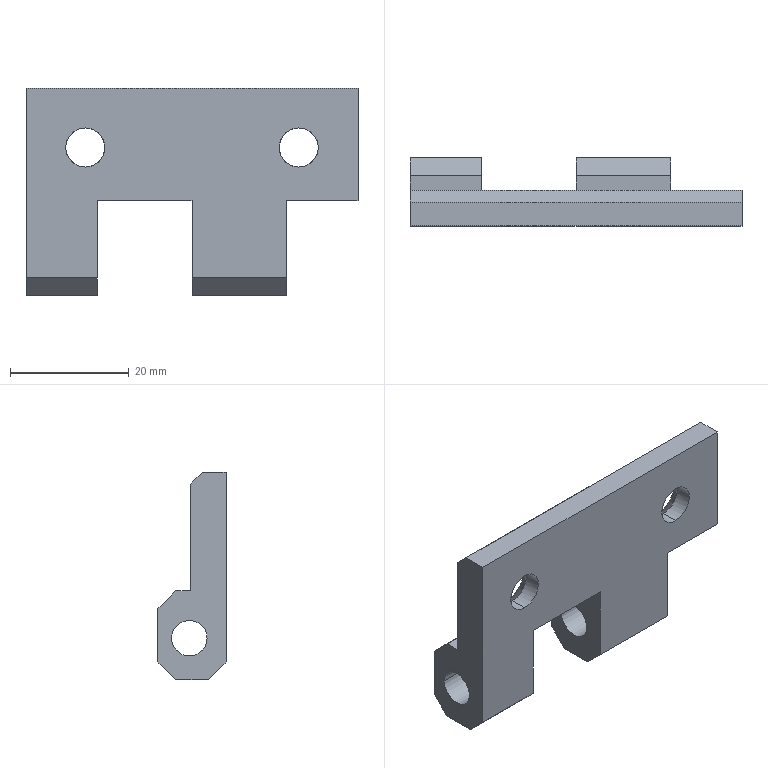Part | NX | features solid 2 | 1 solid | 35 faces | box 56 x 11.5 x 35 mm | volume 9428 mm3 | plane 23 | cylinder 8 | cone 4 | commonest cylinder face diameters 6 x4 6.6 x4
STEP:
#1=CARTESIAN_POINT('',(-668.,-707.,1288.));
#2=VERTEX_POINT('',#1);
#3=CARTESIAN_POINT('',(-668.,-710.,1291.));
#4=VERTEX_POINT('',#3);
#5=CARTESIAN_POINT('',(-668.,-710.,1291.));
#6=DIRECTION('',(0.,-0.7071,0.7071));
#7=VECTOR('',#6,1000.);
#8=LINE('',#5,#7);
#9=EDGE_CURVE('',#2,#4,#8,.T.);
#10=ORIENTED_EDGE('',*,*,#9,.F.);
#11=CARTESIAN_POINT('',(-652.,-707.,1288.));
#12=VERTEX_POINT('',#11);
#13=CARTESIAN_POINT('',(-696.,-707.,1288.));
#14=DIRECTION('',(-1.,0.,0.));
#15=VECTOR('',#14,1000.);
#16=LINE('',#13,#15);
#17=EDGE_CURVE('',#12,#2,#16,.T.);
#18=ORIENTED_EDGE('',*,*,#17,.F.);
#19=CARTESIAN_POINT('',(-652.,-710.,1291.));
#20=VERTEX_POINT('',#19);
#21=CARTESIAN_POINT('',(-652.,-710.,1291.));
#22=DIRECTION('',(0.,0.7071,-0.7071));
#23=VECTOR('',#22,1000.);
#24=LINE('',#21,#23);
#25=EDGE_CURVE('',#20,#12,#24,.T.);
#26=ORIENTED_EDGE('',*,*,#25,.F.);
#27=CARTESIAN_POINT('',(-696.,-710.,1291.));
#28=DIRECTION('',(1.,0.,0.));
#29=VECTOR('',#28,1000.);
#30=LINE('',#27,#29);
#31=EDGE_CURVE('',#4,#20,#30,.T.);
#32=ORIENTED_EDGE('',*,*,#31,.F.);
#33=EDGE_LOOP('',(#10,#18,#26,#32));
#34=FACE_BOUND('',#33,.T.);
#35=CARTESIAN_POINT('',(-696.,-710.,1291.));
#36=DIRECTION('',(0.,0.7071,0.7071));
#37=DIRECTION('',(1.,0.,0.));
#38=AXIS2_PLACEMENT_3D('',#35,#36,#37);
#39=PLANE('',#38);
#40=ADVANCED_FACE('',(#34),#39,.F.);
#41=CARTESIAN_POINT('',(-696.,-707.,1288.));
#42=VERTEX_POINT('',#41);
#43=CARTESIAN_POINT('',(-696.,-710.,1291.));
#44=VERTEX_POINT('',#43);
#45=CARTESIAN_POINT('',(-696.,-710.,1291.));
#46=DIRECTION('',(0.,-0.7071,0.7071));
#47=VECTOR('',#46,1000.);
#48=LINE('',#45,#47);
#49=EDGE_CURVE('',#42,#44,#48,.T.);
#50=ORIENTED_EDGE('',*,*,#49,.F.);
#51=CARTESIAN_POINT('',(-684.,-707.,1288.));
#52=VERTEX_POINT('',#51);
#53=CARTESIAN_POINT('',(-696.,-707.,1288.));
#54=DIRECTION('',(-1.,0.,0.));
#55=VECTOR('',#54,1000.);
#56=LINE('',#53,#55);
#57=EDGE_CURVE('',#52,#42,#56,.T.);
#58=ORIENTED_EDGE('',*,*,#57,.F.);
#59=CARTESIAN_POINT('',(-684.,-710.,1291.));
#60=VERTEX_POINT('',#59);
#61=CARTESIAN_POINT('',(-684.,-710.,1291.));
#62=DIRECTION('',(0.,0.7071,-0.7071));
#63=VECTOR('',#62,1000.);
#64=LINE('',#61,#63);
#65=EDGE_CURVE('',#60,#52,#64,.T.);
#66=ORIENTED_EDGE('',*,*,#65,.F.);
#67=CARTESIAN_POINT('',(-696.,-710.,1291.));
#68=DIRECTION('',(1.,0.,0.));
#69=VECTOR('',#68,1000.);
#70=LINE('',#67,#69);
#71=EDGE_CURVE('',#44,#60,#70,.T.);
#72=ORIENTED_EDGE('',*,*,#71,.F.);
#73=EDGE_LOOP('',(#50,#58,#66,#72));
#74=FACE_BOUND('',#73,.T.);
#75=CARTESIAN_POINT('',(-696.,-710.,1291.));
#76=DIRECTION('',(0.,0.7071,0.7071));
#77=DIRECTION('',(1.,0.,0.));
#78=AXIS2_PLACEMENT_3D('',#75,#76,#77);
#79=PLANE('',#78);
#80=ADVANCED_FACE('',(#74),#79,.F.);
#81=CARTESIAN_POINT('',(-668.,-701.5,1288.));
#82=VERTEX_POINT('',#81);
#83=CARTESIAN_POINT('',(-668.,-698.5,1291.));
#84=VERTEX_POINT('',#83);
#85=CARTESIAN_POINT('',(-668.,-725.516,1263.984));
#86=DIRECTION('',(0.,0.7071,0.7071));
#87=VECTOR('',#86,1000.);
#88=LINE('',#85,#87);
#89=EDGE_CURVE('',#82,#84,#88,.T.);
#90=ORIENTED_EDGE('',*,*,#89,.T.);
#91=CARTESIAN_POINT('',(-652.,-698.5,1291.));
#92=VERTEX_POINT('',#91);
#93=CARTESIAN_POINT('',(-719.032,-698.5,1291.));
#94=DIRECTION('',(1.,0.,0.));
#95=VECTOR('',#94,1000.);
#96=LINE('',#93,#95);
#97=EDGE_CURVE('',#84,#92,#96,.T.);
#98=ORIENTED_EDGE('',*,*,#97,.T.);
#99=CARTESIAN_POINT('',(-652.,-701.5,1288.));
#100=VERTEX_POINT('',#99);
#101=CARTESIAN_POINT('',(-652.,-698.5,1291.));
#102=DIRECTION('',(0.,0.7071,0.7071));
#103=VECTOR('',#102,1000.);
#104=LINE('',#101,#103);
#105=EDGE_CURVE('',#100,#92,#104,.T.);
#106=ORIENTED_EDGE('',*,*,#105,.F.);
#107=CARTESIAN_POINT('',(-696.,-701.5,1288.));
#108=DIRECTION('',(1.,0.,0.));
#109=VECTOR('',#108,1000.);
#110=LINE('',#107,#109);
#111=EDGE_CURVE('',#82,#100,#110,.T.);
#112=ORIENTED_EDGE('',*,*,#111,.F.);
#113=EDGE_LOOP('',(#90,#98,#106,#112));
#114=FACE_BOUND('',#113,.T.);
#115=CARTESIAN_POINT('',(-719.032,-698.5,1291.));
#116=DIRECTION('',(0.,0.7071,-0.7071));
#117=DIRECTION('',(-1.,0.,0.));
#118=AXIS2_PLACEMENT_3D('',#115,#116,#117);
#119=PLANE('',#118);
#120=ADVANCED_FACE('',(#114),#119,.T.);
#121=CARTESIAN_POINT('',(-696.,-701.5,1288.));
#122=VERTEX_POINT('',#121);
#123=CARTESIAN_POINT('',(-696.,-698.5,1291.));
#124=VERTEX_POINT('',#123);
#125=CARTESIAN_POINT('',(-696.,-688.25,1301.25));
#126=DIRECTION('',(0.,0.7071,0.7071));
#127=VECTOR('',#126,1000.);
#128=LINE('',#125,#127);
#129=EDGE_CURVE('',#122,#124,#128,.T.);
#130=ORIENTED_EDGE('',*,*,#129,.T.);
#131=CARTESIAN_POINT('',(-684.,-698.5,1291.));
#132=VERTEX_POINT('',#131);
#133=CARTESIAN_POINT('',(-719.032,-698.5,1291.));
#134=DIRECTION('',(1.,0.,0.));
#135=VECTOR('',#134,1000.);
#136=LINE('',#133,#135);
#137=EDGE_CURVE('',#124,#132,#136,.T.);
#138=ORIENTED_EDGE('',*,*,#137,.T.);
#139=CARTESIAN_POINT('',(-684.,-701.5,1288.));
#140=VERTEX_POINT('',#139);
#141=CARTESIAN_POINT('',(-684.,-733.516,1255.984));
#142=DIRECTION('',(0.,-0.7071,-0.7071));
#143=VECTOR('',#142,1000.);
#144=LINE('',#141,#143);
#145=EDGE_CURVE('',#132,#140,#144,.T.);
#146=ORIENTED_EDGE('',*,*,#145,.T.);
#147=CARTESIAN_POINT('',(-719.032,-701.5,1288.));
#148=DIRECTION('',(1.,0.,0.));
#149=VECTOR('',#148,1000.);
#150=LINE('',#147,#149);
#151=EDGE_CURVE('',#122,#140,#150,.T.);
#152=ORIENTED_EDGE('',*,*,#151,.F.);
#153=EDGE_LOOP('',(#130,#138,#146,#152));
#154=FACE_BOUND('',#153,.T.);
#155=CARTESIAN_POINT('',(-719.032,-698.5,1291.));
#156=DIRECTION('',(0.,0.7071,-0.7071));
#157=DIRECTION('',(-1.,0.,0.));
#158=AXIS2_PLACEMENT_3D('',#155,#156,#157);
#159=PLANE('',#158);
#160=ADVANCED_FACE('',(#154),#159,.T.);
#161=CARTESIAN_POINT('',(-668.,-698.5,1300.));
#162=VERTEX_POINT('',#161);
#163=CARTESIAN_POINT('',(-668.,-701.5,1303.));
#164=VERTEX_POINT('',#163);
#165=CARTESIAN_POINT('',(-668.,-734.016,1335.516));
#166=DIRECTION('',(0.,-0.7071,0.7071));
#167=VECTOR('',#166,1000.);
#168=LINE('',#165,#167);
#169=EDGE_CURVE('',#162,#164,#168,.T.);
#170=ORIENTED_EDGE('',*,*,#169,.T.);
#171=CARTESIAN_POINT('',(-652.,-701.5,1303.));
#172=VERTEX_POINT('',#171);
#173=CARTESIAN_POINT('',(-719.032,-701.5,1303.));
#174=DIRECTION('',(1.,0.,0.));
#175=VECTOR('',#174,1000.);
#176=LINE('',#173,#175);
#177=EDGE_CURVE('',#164,#172,#176,.T.);
#178=ORIENTED_EDGE('',*,*,#177,.T.);
#179=CARTESIAN_POINT('',(-652.,-698.5,1300.));
#180=VERTEX_POINT('',#179);
#181=CARTESIAN_POINT('',(-652.,-701.5,1303.));
#182=DIRECTION('',(0.,-0.7071,0.7071));
#183=VECTOR('',#182,1000.);
#184=LINE('',#181,#183);
#185=EDGE_CURVE('',#180,#172,#184,.T.);
#186=ORIENTED_EDGE('',*,*,#185,.F.);
#187=CARTESIAN_POINT('',(-719.032,-698.5,1300.));
#188=DIRECTION('',(1.,0.,0.));
#189=VECTOR('',#188,1000.);
#190=LINE('',#187,#189);
#191=EDGE_CURVE('',#162,#180,#190,.T.);
#192=ORIENTED_EDGE('',*,*,#191,.F.);
#193=EDGE_LOOP('',(#170,#178,#186,#192));
#194=FACE_BOUND('',#193,.T.);
#195=CARTESIAN_POINT('',(-719.032,-701.5,1303.));
#196=DIRECTION('',(0.,0.7071,0.7071));
#197=DIRECTION('',(1.,0.,0.));
#198=AXIS2_PLACEMENT_3D('',#195,#196,#197);
#199=PLANE('',#198);
#200=ADVANCED_FACE('',(#194),#199,.T.);
#201=CARTESIAN_POINT('',(-696.,-698.5,1300.));
#202=VERTEX_POINT('',#201);
#203=CARTESIAN_POINT('',(-696.,-701.5,1303.));
#204=VERTEX_POINT('',#203);
#205=CARTESIAN_POINT('',(-696.,-715.75,1317.25));
#206=DIRECTION('',(0.,-0.7071,0.7071));
#207=VECTOR('',#206,1000.);
#208=LINE('',#205,#207);
#209=EDGE_CURVE('',#202,#204,#208,.T.);
#210=ORIENTED_EDGE('',*,*,#209,.T.);
#211=CARTESIAN_POINT('',(-684.,-701.5,1303.));
#212=VERTEX_POINT('',#211);
#213=CARTESIAN_POINT('',(-719.032,-701.5,1303.));
#214=DIRECTION('',(1.,0.,0.));
#215=VECTOR('',#214,1000.);
#216=LINE('',#213,#215);
#217=EDGE_CURVE('',#204,#212,#216,.T.);
#218=ORIENTED_EDGE('',*,*,#217,.T.);
#219=CARTESIAN_POINT('',(-684.,-698.5,1300.));
#220=VERTEX_POINT('',#219);
#221=CARTESIAN_POINT('',(-684.,-726.016,1327.516));
#222=DIRECTION('',(0.,0.7071,-0.7071));
#223=VECTOR('',#222,1000.);
#224=LINE('',#221,#223);
#225=EDGE_CURVE('',#212,#220,#224,.T.);
#226=ORIENTED_EDGE('',*,*,#225,.T.);
#227=CARTESIAN_POINT('',(-719.032,-698.5,1300.));
#228=DIRECTION('',(1.,0.,0.));
#229=VECTOR('',#228,1000.);
#230=LINE('',#227,#229);
#231=EDGE_CURVE('',#202,#220,#230,.T.);
#232=ORIENTED_EDGE('',*,*,#231,.F.);
#233=EDGE_LOOP('',(#210,#218,#226,#232));
#234=FACE_BOUND('',#233,.T.);
#235=CARTESIAN_POINT('',(-719.032,-701.5,1303.));
#236=DIRECTION('',(0.,0.7071,0.7071));
#237=DIRECTION('',(1.,0.,0.));
#238=AXIS2_PLACEMENT_3D('',#235,#236,#237);
#239=PLANE('',#238);
#240=ADVANCED_FACE('',(#234),#239,.T.);
#241=CARTESIAN_POINT('',(-684.,-700.8,1295.));
#242=VERTEX_POINT('',#241);
#243=CARTESIAN_POINT('',(-696.,-700.8,1295.));
#244=VERTEX_POINT('',#243);
#245=CARTESIAN_POINT('',(-640.,-700.8,1295.));
#246=DIRECTION('',(-1.,0.,0.));
#247=VECTOR('',#246,1000.);
#248=LINE('',#245,#247);
#249=EDGE_CURVE('',#242,#244,#248,.T.);
#250=ORIENTED_EDGE('',*,*,#249,.F.);
#251=CARTESIAN_POINT('',(-684.,-706.8,1295.));
#252=VERTEX_POINT('',#251);
#253=CARTESIAN_POINT('',(-684.,-703.8,1295.));
#254=DIRECTION('',(-1.,0.,0.));
#255=DIRECTION('',(0.,0.,1.));
#256=AXIS2_PLACEMENT_3D('',#253,#254,#255);
#257=CIRCLE('',#256,3.);
#258=EDGE_CURVE('',#252,#242,#257,.T.);
#259=ORIENTED_EDGE('',*,*,#258,.F.);
#260=CARTESIAN_POINT('',(-696.,-706.8,1295.));
#261=VERTEX_POINT('',#260);
#262=CARTESIAN_POINT('',(-640.,-706.8,1295.));
#263=DIRECTION('',(-1.,0.,0.));
#264=VECTOR('',#263,1000.);
#265=LINE('',#262,#264);
#266=EDGE_CURVE('',#261,#252,#265,.F.);
#267=ORIENTED_EDGE('',*,*,#266,.F.);
#268=CARTESIAN_POINT('',(-696.,-703.8,1295.));
#269=DIRECTION('',(1.,0.,0.));
#270=DIRECTION('',(0.,-1.,0.));
#271=AXIS2_PLACEMENT_3D('',#268,#269,#270);
#272=CIRCLE('',#271,3.);
#273=EDGE_CURVE('',#244,#261,#272,.T.);
#274=ORIENTED_EDGE('',*,*,#273,.F.);
#275=EDGE_LOOP('',(#250,#259,#267,#274));
#276=FACE_BOUND('',#275,.T.);
#277=CARTESIAN_POINT('',(-640.,-703.8,1295.));
#278=DIRECTION('',(-1.,0.,0.));
#279=DIRECTION('',(0.,-1.,0.));
#280=AXIS2_PLACEMENT_3D('',#277,#278,#279);
#281=CYLINDRICAL_SURFACE('',#280,3.);
#282=ADVANCED_FACE('',(#276),#281,.F.);
#283=CARTESIAN_POINT('',(-668.,-700.8,1295.));
#284=VERTEX_POINT('',#283);
#285=CARTESIAN_POINT('',(-652.,-700.8,1295.));
#286=VERTEX_POINT('',#285);
#287=CARTESIAN_POINT('',(-640.,-700.8,1295.));
#288=DIRECTION('',(-1.,0.,0.));
#289=VECTOR('',#288,1000.);
#290=LINE('',#287,#289);
#291=EDGE_CURVE('',#284,#286,#290,.F.);
#292=ORIENTED_EDGE('',*,*,#291,.T.);
#293=CARTESIAN_POINT('',(-652.,-706.8,1295.));
#294=VERTEX_POINT('',#293);
#295=CARTESIAN_POINT('',(-652.,-703.8,1295.));
#296=DIRECTION('',(-1.,0.,0.));
#297=DIRECTION('',(0.,0.,1.));
#298=AXIS2_PLACEMENT_3D('',#295,#296,#297);
#299=CIRCLE('',#298,3.);
#300=EDGE_CURVE('',#294,#286,#299,.T.);
#301=ORIENTED_EDGE('',*,*,#300,.F.);
#302=CARTESIAN_POINT('',(-668.,-706.8,1295.));
#303=VERTEX_POINT('',#302);
#304=CARTESIAN_POINT('',(-640.,-706.8,1295.));
#305=DIRECTION('',(-1.,0.,0.));
#306=VECTOR('',#305,1000.);
#307=LINE('',#304,#306);
#308=EDGE_CURVE('',#294,#303,#307,.T.);
#309=ORIENTED_EDGE('',*,*,#308,.T.);
#310=CARTESIAN_POINT('',(-668.,-703.8,1295.));
#311=DIRECTION('',(1.,0.,0.));
#312=DIRECTION('',(0.,-1.,0.));
#313=AXIS2_PLACEMENT_3D('',#310,#311,#312);
#314=CIRCLE('',#313,3.);
#315=EDGE_CURVE('',#284,#303,#314,.T.);
#316=ORIENTED_EDGE('',*,*,#315,.F.);
#317=EDGE_LOOP('',(#292,#301,#309,#316));
#318=FACE_BOUND('',#317,.T.);
#319=CARTESIAN_POINT('',(-640.,-703.8,1295.));
#320=DIRECTION('',(-1.,0.,0.));
#321=DIRECTION('',(0.,-1.,0.));
#322=AXIS2_PLACEMENT_3D('',#319,#320,#321);
#323=CYLINDRICAL_SURFACE('',#322,3.);
#324=ADVANCED_FACE('',(#318),#323,.F.);
#325=CARTESIAN_POINT('',(-668.,-710.,1304.));
#326=VERTEX_POINT('',#325);
#327=CARTESIAN_POINT('',(-684.,-710.,1304.));
#328=VERTEX_POINT('',#327);
#329=CARTESIAN_POINT('',(-696.,-710.,1304.));
#330=DIRECTION('',(-1.,0.,0.));
#331=VECTOR('',#330,1000.);
#332=LINE('',#329,#331);
#333=EDGE_CURVE('',#326,#328,#332,.T.);
#334=ORIENTED_EDGE('',*,*,#333,.T.);
#335=CARTESIAN_POINT('',(-684.,-704.,1304.));
#336=VERTEX_POINT('',#335);
#337=CARTESIAN_POINT('',(-684.,-765.532,1304.));
#338=DIRECTION('',(0.,1.,0.));
#339=VECTOR('',#338,1000.);
#340=LINE('',#337,#339);
#341=EDGE_CURVE('',#328,#336,#340,.T.);
#342=ORIENTED_EDGE('',*,*,#341,.T.);
#343=CARTESIAN_POINT('',(-668.,-704.,1304.));
#344=VERTEX_POINT('',#343);
#345=CARTESIAN_POINT('',(-696.,-704.,1304.));
#346=DIRECTION('',(1.,0.,0.));
#347=VECTOR('',#346,1000.);
#348=LINE('',#345,#347);
#349=EDGE_CURVE('',#336,#344,#348,.T.);
#350=ORIENTED_EDGE('',*,*,#349,.T.);
#351=CARTESIAN_POINT('',(-668.,-765.532,1304.));
#352=DIRECTION('',(0.,1.,0.));
#353=VECTOR('',#352,1000.);
#354=LINE('',#351,#353);
#355=EDGE_CURVE('',#326,#344,#354,.T.);
#356=ORIENTED_EDGE('',*,*,#355,.F.);
#357=EDGE_LOOP('',(#334,#342,#350,#356));
#358=FACE_BOUND('',#357,.T.);
#359=CARTESIAN_POINT('',(-684.,-765.532,1304.));
#360=DIRECTION('',(0.,0.,1.));
#361=DIRECTION('',(1.,0.,0.));
#362=AXIS2_PLACEMENT_3D('',#359,#360,#361);
#363=PLANE('',#362);
#364=ADVANCED_FACE('',(#358),#363,.F.);
#365=CARTESIAN_POINT('',(-640.,-710.,1304.));
#366=VERTEX_POINT('',#365);
#367=CARTESIAN_POINT('',(-652.,-710.,1304.));
#368=VERTEX_POINT('',#367);
#369=CARTESIAN_POINT('',(-696.,-710.,1304.));
#370=DIRECTION('',(-1.,0.,0.));
#371=VECTOR('',#370,1000.);
#372=LINE('',#369,#371);
#373=EDGE_CURVE('',#366,#368,#372,.T.);
#374=ORIENTED_EDGE('',*,*,#373,.T.);
#375=CARTESIAN_POINT('',(-652.,-704.,1304.));
#376=VERTEX_POINT('',#375);
#377=CARTESIAN_POINT('',(-652.,-765.532,1304.));
#378=DIRECTION('',(0.,1.,0.));
#379=VECTOR('',#378,1000.);
#380=LINE('',#377,#379);
#381=EDGE_CURVE('',#368,#376,#380,.T.);
#382=ORIENTED_EDGE('',*,*,#381,.T.);
#383=CARTESIAN_POINT('',(-640.,-704.,1304.));
#384=VERTEX_POINT('',#383);
#385=CARTESIAN_POINT('',(-696.,-704.,1304.));
#386=DIRECTION('',(1.,0.,0.));
#387=VECTOR('',#386,1000.);
#388=LINE('',#385,#387);
#389=EDGE_CURVE('',#376,#384,#388,.T.);
#390=ORIENTED_EDGE('',*,*,#389,.T.);
#391=CARTESIAN_POINT('',(-640.,-710.,1304.));
#392=DIRECTION('',(0.,-1.,0.));
#393=VECTOR('',#392,1000.);
#394=LINE('',#391,#393);
#395=EDGE_CURVE('',#384,#366,#394,.T.);
#396=ORIENTED_EDGE('',*,*,#395,.T.);
#397=EDGE_LOOP('',(#374,#382,#390,#396));
#398=FACE_BOUND('',#397,.T.);
#399=CARTESIAN_POINT('',(-652.,-765.532,1304.));
#400=DIRECTION('',(0.,0.,1.));
#401=DIRECTION('',(1.,0.,0.));
#402=AXIS2_PLACEMENT_3D('',#399,#400,#401);
#403=PLANE('',#402);
#404=ADVANCED_FACE('',(#398),#403,.F.);
#405=CARTESIAN_POINT('',(-679.6,-704.,1313.));
#406=VERTEX_POINT('',#405);
#407=CARTESIAN_POINT('',(-682.7,-707.1,1313.));
#408=VERTEX_POINT('',#407);
#409=CARTESIAN_POINT('',(-679.6,-704.,1313.));
#410=DIRECTION('',(0.7071,0.7071,0.));
#411=VECTOR('',#410,1000.);
#412=LINE('',#409,#411);
#413=EDGE_CURVE('',#406,#408,#412,.F.);
#414=ORIENTED_EDGE('',*,*,#413,.T.);
#415=CARTESIAN_POINT('',(-686.,-707.1,1316.3));
#416=VERTEX_POINT('',#415);
#417=CARTESIAN_POINT('',(-686.,-707.1,1313.));
#418=DIRECTION('',(0.,1.,0.));
#419=DIRECTION('',(-1.,0.,0.));
#420=AXIS2_PLACEMENT_3D('',#417,#418,#419);
#421=CIRCLE('',#420,3.3);
#422=EDGE_CURVE('',#416,#408,#421,.T.);
#423=ORIENTED_EDGE('',*,*,#422,.F.);
#424=CARTESIAN_POINT('',(-689.3,-707.1,1313.));
#425=VERTEX_POINT('',#424);
#426=CARTESIAN_POINT('',(-686.,-707.1,1313.));
#427=DIRECTION('',(0.,1.,0.));
#428=DIRECTION('',(-1.,0.,0.));
#429=AXIS2_PLACEMENT_3D('',#426,#427,#428);
#430=CIRCLE('',#429,3.3);
#431=EDGE_CURVE('',#425,#416,#430,.T.);
#432=ORIENTED_EDGE('',*,*,#431,.F.);
#433=CARTESIAN_POINT('',(-692.4,-704.,1313.));
#434=VERTEX_POINT('',#433);
#435=CARTESIAN_POINT('',(-692.4,-704.,1313.));
#436=DIRECTION('',(-0.7071,0.7071,0.));
#437=VECTOR('',#436,1000.);
#438=LINE('',#435,#437);
#439=EDGE_CURVE('',#425,#434,#438,.T.);
#440=ORIENTED_EDGE('',*,*,#439,.T.);
#441=CARTESIAN_POINT('',(-686.,-704.,1313.));
#442=DIRECTION('',(0.,-1.,0.));
#443=DIRECTION('',(-1.,0.,0.));
#444=AXIS2_PLACEMENT_3D('',#441,#442,#443);
#445=CIRCLE('',#444,6.4);
#446=EDGE_CURVE('',#406,#434,#445,.T.);
#447=ORIENTED_EDGE('',*,*,#446,.F.);
#448=EDGE_LOOP('',(#414,#423,#432,#440,#447));
#449=FACE_BOUND('',#448,.T.);
#450=CARTESIAN_POINT('',(-686.,-704.,1313.));
#451=DIRECTION('',(0.,1.,0.));
#452=DIRECTION('',(-1.,0.,0.));
#453=AXIS2_PLACEMENT_3D('',#450,#451,#452);
#454=CONICAL_SURFACE('',#453,6.4,0.7854);
#455=ADVANCED_FACE('',(#449),#454,.F.);
#456=CARTESIAN_POINT('',(-686.,-710.,1316.3));
#457=VERTEX_POINT('',#456);
#458=CARTESIAN_POINT('',(-686.,-774.132,1316.3));
#459=DIRECTION('',(0.,1.,0.));
#460=VECTOR('',#459,1000.);
#461=LINE('',#458,#460);
#462=EDGE_CURVE('',#457,#416,#461,.T.);
#463=ORIENTED_EDGE('',*,*,#462,.F.);
#464=CARTESIAN_POINT('',(-686.,-710.,1309.7));
#465=VERTEX_POINT('',#464);
#466=CARTESIAN_POINT('',(-686.,-710.,1313.));
#467=DIRECTION('',(0.,-1.,0.));
#468=DIRECTION('',(0.,0.,1.));
#469=AXIS2_PLACEMENT_3D('',#466,#467,#468);
#470=CIRCLE('',#469,3.3);
#471=EDGE_CURVE('',#457,#465,#470,.T.);
#472=ORIENTED_EDGE('',*,*,#471,.T.);
#473=CARTESIAN_POINT('',(-686.,-707.1,1309.7));
#474=VERTEX_POINT('',#473);
#475=CARTESIAN_POINT('',(-686.,-774.132,1309.7));
#476=DIRECTION('',(0.,1.,0.));
#477=VECTOR('',#476,1000.);
#478=LINE('',#475,#477);
#479=EDGE_CURVE('',#474,#465,#478,.F.);
#480=ORIENTED_EDGE('',*,*,#479,.F.);
#481=CARTESIAN_POINT('',(-686.,-707.1,1313.));
#482=DIRECTION('',(0.,1.,0.));
#483=DIRECTION('',(-1.,0.,0.));
#484=AXIS2_PLACEMENT_3D('',#481,#482,#483);
#485=CIRCLE('',#484,3.3);
#486=EDGE_CURVE('',#474,#425,#485,.T.);
#487=ORIENTED_EDGE('',*,*,#486,.T.);
#488=ORIENTED_EDGE('',*,*,#431,.T.);
#489=EDGE_LOOP('',(#463,#472,#480,#487,#488));
#490=FACE_BOUND('',#489,.T.);
#491=CARTESIAN_POINT('',(-686.,-774.132,1313.));
#492=DIRECTION('',(0.,1.,0.));
#493=DIRECTION('',(0.,0.,-1.));
#494=AXIS2_PLACEMENT_3D('',#491,#492,#493);
#495=CYLINDRICAL_SURFACE('',#494,3.3);
#496=ADVANCED_FACE('',(#490),#495,.F.);
#497=CARTESIAN_POINT('',(-646.7,-707.1,1313.));
#498=VERTEX_POINT('',#497);
#499=CARTESIAN_POINT('',(-643.6,-704.,1313.));
#500=VERTEX_POINT('',#499);
#501=CARTESIAN_POINT('',(-643.6,-704.,1313.));
#502=DIRECTION('',(0.7071,0.7071,0.));
#503=VECTOR('',#502,1000.);
#504=LINE('',#501,#503);
#505=EDGE_CURVE('',#498,#500,#504,.T.);
#506=ORIENTED_EDGE('',*,*,#505,.F.);
#507=CARTESIAN_POINT('',(-650.,-707.1,1316.3));
#508=VERTEX_POINT('',#507);
#509=CARTESIAN_POINT('',(-650.,-707.1,1313.));
#510=DIRECTION('',(0.,1.,0.));
#511=DIRECTION('',(-1.,0.,0.));
#512=AXIS2_PLACEMENT_3D('',#509,#510,#511);
#513=CIRCLE('',#512,3.3);
#514=EDGE_CURVE('',#508,#498,#513,.T.);
#515=ORIENTED_EDGE('',*,*,#514,.F.);
#516=CARTESIAN_POINT('',(-653.3,-707.1,1313.));
#517=VERTEX_POINT('',#516);
#518=CARTESIAN_POINT('',(-650.,-707.1,1313.));
#519=DIRECTION('',(0.,1.,0.));
#520=DIRECTION('',(-1.,0.,0.));
#521=AXIS2_PLACEMENT_3D('',#518,#519,#520);
#522=CIRCLE('',#521,3.3);
#523=EDGE_CURVE('',#517,#508,#522,.T.);
#524=ORIENTED_EDGE('',*,*,#523,.F.);
#525=CARTESIAN_POINT('',(-656.4,-704.,1313.));
#526=VERTEX_POINT('',#525);
#527=CARTESIAN_POINT('',(-656.4,-704.,1313.));
#528=DIRECTION('',(-0.7071,0.7071,0.));
#529=VECTOR('',#528,1000.);
#530=LINE('',#527,#529);
#531=EDGE_CURVE('',#526,#517,#530,.F.);
#532=ORIENTED_EDGE('',*,*,#531,.F.);
#533=CARTESIAN_POINT('',(-650.,-704.,1313.));
#534=DIRECTION('',(0.,-1.,0.));
#535=DIRECTION('',(-1.,0.,0.));
#536=AXIS2_PLACEMENT_3D('',#533,#534,#535);
#537=CIRCLE('',#536,6.4);
#538=EDGE_CURVE('',#500,#526,#537,.T.);
#539=ORIENTED_EDGE('',*,*,#538,.F.);
#540=EDGE_LOOP('',(#506,#515,#524,#532,#539));
#541=FACE_BOUND('',#540,.T.);
#542=CARTESIAN_POINT('',(-650.,-704.,1313.));
#543=DIRECTION('',(0.,1.,0.));
#544=DIRECTION('',(-1.,0.,0.));
#545=AXIS2_PLACEMENT_3D('',#542,#543,#544);
#546=CONICAL_SURFACE('',#545,6.4,0.7854);
#547=ADVANCED_FACE('',(#541),#546,.F.);
#548=CARTESIAN_POINT('',(-650.,-710.,1316.3));
#549=VERTEX_POINT('',#548);
#550=CARTESIAN_POINT('',(-650.,-774.132,1316.3));
#551=DIRECTION('',(0.,1.,0.));
#552=VECTOR('',#551,1000.);
#553=LINE('',#550,#552);
#554=EDGE_CURVE('',#549,#508,#553,.T.);
#555=ORIENTED_EDGE('',*,*,#554,.F.);
#556=CARTESIAN_POINT('',(-650.,-710.,1309.7));
#557=VERTEX_POINT('',#556);
#558=CARTESIAN_POINT('',(-650.,-710.,1313.));
#559=DIRECTION('',(0.,-1.,0.));
#560=DIRECTION('',(0.,0.,1.));
#561=AXIS2_PLACEMENT_3D('',#558,#559,#560);
#562=CIRCLE('',#561,3.3);
#563=EDGE_CURVE('',#549,#557,#562,.T.);
#564=ORIENTED_EDGE('',*,*,#563,.T.);
#565=CARTESIAN_POINT('',(-650.,-707.1,1309.7));
#566=VERTEX_POINT('',#565);
#567=CARTESIAN_POINT('',(-650.,-774.132,1309.7));
#568=DIRECTION('',(0.,1.,0.));
#569=VECTOR('',#568,1000.);
#570=LINE('',#567,#569);
#571=EDGE_CURVE('',#566,#557,#570,.F.);
#572=ORIENTED_EDGE('',*,*,#571,.F.);
#573=CARTESIAN_POINT('',(-650.,-707.1,1313.));
#574=DIRECTION('',(0.,1.,0.));
#575=DIRECTION('',(-1.,0.,0.));
#576=AXIS2_PLACEMENT_3D('',#573,#574,#575);
#577=CIRCLE('',#576,3.3);
#578=EDGE_CURVE('',#566,#517,#577,.T.);
#579=ORIENTED_EDGE('',*,*,#578,.T.);
#580=ORIENTED_EDGE('',*,*,#523,.T.);
#581=EDGE_LOOP('',(#555,#564,#572,#579,#580));
#582=FACE_BOUND('',#581,.T.);
#583=CARTESIAN_POINT('',(-650.,-774.132,1313.));
#584=DIRECTION('',(0.,1.,0.));
#585=DIRECTION('',(0.,0.,-1.));
#586=AXIS2_PLACEMENT_3D('',#583,#584,#585);
#587=CYLINDRICAL_SURFACE('',#586,3.3);
#588=ADVANCED_FACE('',(#582),#587,.F.);
#589=ORIENTED_EDGE('',*,*,#395,.F.);
#590=CARTESIAN_POINT('',(-640.,-704.,1321.));
#591=VERTEX_POINT('',#590);
#592=CARTESIAN_POINT('',(-640.,-704.,1303.));
#593=DIRECTION('',(0.,0.,1.));
#594=VECTOR('',#593,1000.);
#595=LINE('',#592,#594);
#596=EDGE_CURVE('',#384,#591,#595,.T.);
#597=ORIENTED_EDGE('',*,*,#596,.T.);
#598=CARTESIAN_POINT('',(-640.,-706.,1323.));
#599=VERTEX_POINT('',#598);
#600=CARTESIAN_POINT('',(-640.,-704.,1321.));
#601=DIRECTION('',(0.,-0.7071,0.7071));
#602=VECTOR('',#601,1000.);
#603=LINE('',#600,#602);
#604=EDGE_CURVE('',#591,#599,#603,.T.);
#605=ORIENTED_EDGE('',*,*,#604,.T.);
#606=CARTESIAN_POINT('',(-640.,-710.,1323.));
#607=VERTEX_POINT('',#606);
#608=CARTESIAN_POINT('',(-640.,-706.,1323.));
#609=DIRECTION('',(0.,-1.,0.));
#610=VECTOR('',#609,1000.);
#611=LINE('',#608,#610);
#612=EDGE_CURVE('',#599,#607,#611,.T.);
#613=ORIENTED_EDGE('',*,*,#612,.T.);
#614=CARTESIAN_POINT('',(-640.,-710.,1323.));
#615=DIRECTION('',(0.,0.,-1.));
#616=VECTOR('',#615,1000.);
#617=LINE('',#614,#616);
#618=EDGE_CURVE('',#607,#366,#617,.T.);
#619=ORIENTED_EDGE('',*,*,#618,.T.);
#620=EDGE_LOOP('',(#589,#597,#605,#613,#619));
#621=FACE_BOUND('',#620,.T.);
#622=CARTESIAN_POINT('',(-640.,-710.,1323.));
#623=DIRECTION('',(1.,0.,0.));
#624=DIRECTION('',(0.,0.,1.));
#625=AXIS2_PLACEMENT_3D('',#622,#623,#624);
#626=PLANE('',#625);
#627=ADVANCED_FACE('',(#621),#626,.T.);
#628=ORIENTED_EDGE('',*,*,#604,.F.);
#629=CARTESIAN_POINT('',(-696.,-704.,1321.));
#630=VERTEX_POINT('',#629);
#631=CARTESIAN_POINT('',(-696.,-704.,1321.));
#632=DIRECTION('',(1.,0.,0.));
#633=VECTOR('',#632,1000.);
#634=LINE('',#631,#633);
#635=EDGE_CURVE('',#630,#591,#634,.T.);
#636=ORIENTED_EDGE('',*,*,#635,.F.);
#637=CARTESIAN_POINT('',(-696.,-706.,1323.));
#638=VERTEX_POINT('',#637);
#639=CARTESIAN_POINT('',(-696.,-704.,1321.));
#640=DIRECTION('',(0.,-0.7071,0.7071));
#641=VECTOR('',#640,1000.);
#642=LINE('',#639,#641);
#643=EDGE_CURVE('',#630,#638,#642,.T.);
#644=ORIENTED_EDGE('',*,*,#643,.T.);
#645=CARTESIAN_POINT('',(-696.,-706.,1323.));
#646=DIRECTION('',(1.,0.,0.));
#647=VECTOR('',#646,1000.);
#648=LINE('',#645,#647);
#649=EDGE_CURVE('',#638,#599,#648,.T.);
#650=ORIENTED_EDGE('',*,*,#649,.T.);
#651=EDGE_LOOP('',(#628,#636,#644,#650));
#652=FACE_BOUND('',#651,.T.);
#653=CARTESIAN_POINT('',(-696.,-704.,1321.));
#654=DIRECTION('',(0.,0.7071,0.7071));
#655=DIRECTION('',(1.,0.,0.));
#656=AXIS2_PLACEMENT_3D('',#653,#654,#655);
#657=PLANE('',#656);
#658=ADVANCED_FACE('',(#652),#657,.T.);
#659=CARTESIAN_POINT('',(-650.,-704.,1313.));
#660=DIRECTION('',(0.,-1.,0.));
#661=DIRECTION('',(-1.,0.,0.));
#662=AXIS2_PLACEMENT_3D('',#659,#660,#661);
#663=CIRCLE('',#662,6.4);
#664=EDGE_CURVE('',#526,#500,#663,.T.);
#665=ORIENTED_EDGE('',*,*,#664,.T.);
#666=ORIENTED_EDGE('',*,*,#538,.T.);
#667=EDGE_LOOP('',(#665,#666));
#668=FACE_BOUND('',#667,.T.);
#669=CARTESIAN_POINT('',(-686.,-704.,1313.));
#670=DIRECTION('',(0.,-1.,0.));
#671=DIRECTION('',(-1.,0.,0.));
#672=AXIS2_PLACEMENT_3D('',#669,#670,#671);
#673=CIRCLE('',#672,6.4);
#674=EDGE_CURVE('',#434,#406,#673,.T.);
#675=ORIENTED_EDGE('',*,*,#674,.T.);
#676=ORIENTED_EDGE('',*,*,#446,.T.);
#677=EDGE_LOOP('',(#675,#676));
#678=FACE_BOUND('',#677,.T.);
#679=CARTESIAN_POINT('',(-684.,-704.,1303.));
#680=VERTEX_POINT('',#679);
#681=CARTESIAN_POINT('',(-684.,-704.,1303.));
#682=DIRECTION('',(0.,0.,1.));
#683=VECTOR('',#682,1000.);
#684=LINE('',#681,#683);
#685=EDGE_CURVE('',#680,#336,#684,.T.);
#686=ORIENTED_EDGE('',*,*,#685,.F.);
#687=CARTESIAN_POINT('',(-696.,-704.,1303.));
#688=VERTEX_POINT('',#687);
#689=CARTESIAN_POINT('',(-696.,-704.,1303.));
#690=DIRECTION('',(1.,0.,0.));
#691=VECTOR('',#690,1000.);
#692=LINE('',#689,#691);
#693=EDGE_CURVE('',#688,#680,#692,.T.);
#694=ORIENTED_EDGE('',*,*,#693,.F.);
#695=CARTESIAN_POINT('',(-696.,-704.,1303.));
#696=DIRECTION('',(0.,0.,1.));
#697=VECTOR('',#696,1000.);
#698=LINE('',#695,#697);
#699=EDGE_CURVE('',#688,#630,#698,.T.);
#700=ORIENTED_EDGE('',*,*,#699,.T.);
#701=ORIENTED_EDGE('',*,*,#635,.T.);
#702=ORIENTED_EDGE('',*,*,#596,.F.);
#703=ORIENTED_EDGE('',*,*,#389,.F.);
#704=CARTESIAN_POINT('',(-652.,-704.,1303.));
#705=VERTEX_POINT('',#704);
#706=CARTESIAN_POINT('',(-652.,-704.,1303.));
#707=DIRECTION('',(0.,0.,1.));
#708=VECTOR('',#707,1000.);
#709=LINE('',#706,#708);
#710=EDGE_CURVE('',#705,#376,#709,.T.);
#711=ORIENTED_EDGE('',*,*,#710,.F.);
#712=CARTESIAN_POINT('',(-668.,-704.,1303.));
#713=VERTEX_POINT('',#712);
#714=CARTESIAN_POINT('',(-696.,-704.,1303.));
#715=DIRECTION('',(1.,0.,0.));
#716=VECTOR('',#715,1000.);
#717=LINE('',#714,#716);
#718=EDGE_CURVE('',#713,#705,#717,.T.);
#719=ORIENTED_EDGE('',*,*,#718,.F.);
#720=CARTESIAN_POINT('',(-668.,-704.,1303.));
#721=DIRECTION('',(0.,0.,-1.));
#722=VECTOR('',#721,1000.);
#723=LINE('',#720,#722);
#724=EDGE_CURVE('',#344,#713,#723,.T.);
#725=ORIENTED_EDGE('',*,*,#724,.F.);
#726=ORIENTED_EDGE('',*,*,#349,.F.);
#727=EDGE_LOOP('',(#686,#694,#700,#701,#702,#703,#711,#719,#725,#726));
#728=FACE_BOUND('',#727,.T.);
#729=CARTESIAN_POINT('',(-696.,-704.,1303.));
#730=DIRECTION('',(0.,1.,0.));
#731=DIRECTION('',(1.,0.,0.));
#732=AXIS2_PLACEMENT_3D('',#729,#730,#731);
#733=PLANE('',#732);
#734=ADVANCED_FACE('',(#668,#678,#728),#733,.T.);
#735=CARTESIAN_POINT('',(-650.,-710.,1313.));
#736=DIRECTION('',(0.,-1.,0.));
#737=DIRECTION('',(0.,0.,1.));
#738=AXIS2_PLACEMENT_3D('',#735,#736,#737);
#739=CIRCLE('',#738,3.3);
#740=EDGE_CURVE('',#557,#549,#739,.T.);
#741=ORIENTED_EDGE('',*,*,#740,.F.);
#742=ORIENTED_EDGE('',*,*,#563,.F.);
#743=EDGE_LOOP('',(#741,#742));
#744=FACE_BOUND('',#743,.T.);
#745=CARTESIAN_POINT('',(-686.,-710.,1313.));
#746=DIRECTION('',(0.,-1.,0.));
#747=DIRECTION('',(0.,0.,1.));
#748=AXIS2_PLACEMENT_3D('',#745,#746,#747);
#749=CIRCLE('',#748,3.3);
#750=EDGE_CURVE('',#465,#457,#749,.T.);
#751=ORIENTED_EDGE('',*,*,#750,.F.);
#752=ORIENTED_EDGE('',*,*,#471,.F.);
#753=EDGE_LOOP('',(#751,#752));
#754=FACE_BOUND('',#753,.T.);
#755=CARTESIAN_POINT('',(-696.,-710.,1323.));
#756=VERTEX_POINT('',#755);
#757=CARTESIAN_POINT('',(-696.,-710.,1323.));
#758=DIRECTION('',(0.,0.,-1.));
#759=VECTOR('',#758,1000.);
#760=LINE('',#757,#759);
#761=EDGE_CURVE('',#756,#44,#760,.T.);
#762=ORIENTED_EDGE('',*,*,#761,.T.);
#763=ORIENTED_EDGE('',*,*,#71,.T.);
#764=CARTESIAN_POINT('',(-684.,-710.,1323.));
#765=DIRECTION('',(0.,0.,-1.));
#766=VECTOR('',#765,1000.);
#767=LINE('',#764,#766);
#768=EDGE_CURVE('',#328,#60,#767,.T.);
#769=ORIENTED_EDGE('',*,*,#768,.F.);
#770=ORIENTED_EDGE('',*,*,#333,.F.);
#771=CARTESIAN_POINT('',(-668.,-710.,1323.));
#772=DIRECTION('',(0.,0.,1.));
#773=VECTOR('',#772,1000.);
#774=LINE('',#771,#773);
#775=EDGE_CURVE('',#4,#326,#774,.T.);
#776=ORIENTED_EDGE('',*,*,#775,.F.);
#777=ORIENTED_EDGE('',*,*,#31,.T.);
#778=CARTESIAN_POINT('',(-652.,-710.,1323.));
#779=DIRECTION('',(0.,0.,-1.));
#780=VECTOR('',#779,1000.);
#781=LINE('',#778,#780);
#782=EDGE_CURVE('',#368,#20,#781,.T.);
#783=ORIENTED_EDGE('',*,*,#782,.F.);
#784=ORIENTED_EDGE('',*,*,#373,.F.);
#785=ORIENTED_EDGE('',*,*,#618,.F.);
#786=CARTESIAN_POINT('',(-696.,-710.,1323.));
#787=DIRECTION('',(1.,0.,0.));
#788=VECTOR('',#787,1000.);
#789=LINE('',#786,#788);
#790=EDGE_CURVE('',#756,#607,#789,.T.);
#791=ORIENTED_EDGE('',*,*,#790,.F.);
#792=EDGE_LOOP('',(#762,#763,#769,#770,#776,#777,#783,#784,#785,#791));
#793=FACE_BOUND('',#792,.T.);
#794=CARTESIAN_POINT('',(-696.,-710.,1323.));
#795=DIRECTION('',(0.,-1.,0.));
#796=DIRECTION('',(-1.,0.,0.));
#797=AXIS2_PLACEMENT_3D('',#794,#795,#796);
#798=PLANE('',#797);
#799=ADVANCED_FACE('',(#744,#754,#793),#798,.T.);
#800=ORIENTED_EDGE('',*,*,#612,.F.);
#801=ORIENTED_EDGE('',*,*,#649,.F.);
#802=CARTESIAN_POINT('',(-696.,-706.,1323.));
#803=DIRECTION('',(0.,-1.,0.));
#804=VECTOR('',#803,1000.);
#805=LINE('',#802,#804);
#806=EDGE_CURVE('',#638,#756,#805,.T.);
#807=ORIENTED_EDGE('',*,*,#806,.T.);
#808=ORIENTED_EDGE('',*,*,#790,.T.);
#809=EDGE_LOOP('',(#800,#801,#807,#808));
#810=FACE_BOUND('',#809,.T.);
#811=CARTESIAN_POINT('',(-696.,-706.,1323.));
#812=DIRECTION('',(0.,0.,1.));
#813=DIRECTION('',(1.,0.,0.));
#814=AXIS2_PLACEMENT_3D('',#811,#812,#813);
#815=PLANE('',#814);
#816=ADVANCED_FACE('',(#810),#815,.T.);
#817=CARTESIAN_POINT('',(-652.,-698.5,1303.));
#818=DIRECTION('',(0.,-1.,0.));
#819=VECTOR('',#818,1000.);
#820=LINE('',#817,#819);
#821=EDGE_CURVE('',#172,#705,#820,.T.);
#822=ORIENTED_EDGE('',*,*,#821,.F.);
#823=ORIENTED_EDGE('',*,*,#177,.F.);
#824=CARTESIAN_POINT('',(-668.,-698.5,1303.));
#825=DIRECTION('',(0.,1.,0.));
#826=VECTOR('',#825,1000.);
#827=LINE('',#824,#826);
#828=EDGE_CURVE('',#713,#164,#827,.T.);
#829=ORIENTED_EDGE('',*,*,#828,.F.);
#830=ORIENTED_EDGE('',*,*,#718,.T.);
#831=EDGE_LOOP('',(#822,#823,#829,#830));
#832=FACE_BOUND('',#831,.T.);
#833=CARTESIAN_POINT('',(-696.,-698.5,1303.));
#834=DIRECTION('',(0.,0.,1.));
#835=DIRECTION('',(1.,0.,0.));
#836=AXIS2_PLACEMENT_3D('',#833,#834,#835);
#837=PLANE('',#836);
#838=ADVANCED_FACE('',(#832),#837,.T.);
#839=CARTESIAN_POINT('',(-684.,-698.5,1303.));
#840=DIRECTION('',(0.,-1.,0.));
#841=VECTOR('',#840,1000.);
#842=LINE('',#839,#841);
#843=EDGE_CURVE('',#212,#680,#842,.T.);
#844=ORIENTED_EDGE('',*,*,#843,.F.);
#845=ORIENTED_EDGE('',*,*,#217,.F.);
#846=CARTESIAN_POINT('',(-696.,-698.5,1303.));
#847=DIRECTION('',(0.,-1.,0.));
#848=VECTOR('',#847,1000.);
#849=LINE('',#846,#848);
#850=EDGE_CURVE('',#204,#688,#849,.T.);
#851=ORIENTED_EDGE('',*,*,#850,.T.);
#852=ORIENTED_EDGE('',*,*,#693,.T.);
#853=EDGE_LOOP('',(#844,#845,#851,#852));
#854=FACE_BOUND('',#853,.T.);
#855=CARTESIAN_POINT('',(-696.,-698.5,1303.));
#856=DIRECTION('',(0.,0.,1.));
#857=DIRECTION('',(1.,0.,0.));
#858=AXIS2_PLACEMENT_3D('',#855,#856,#857);
#859=PLANE('',#858);
#860=ADVANCED_FACE('',(#854),#859,.T.);
#861=CARTESIAN_POINT('',(-652.,-765.532,1288.));
#862=DIRECTION('',(0.,1.,0.));
#863=VECTOR('',#862,1000.);
#864=LINE('',#861,#863);
#865=EDGE_CURVE('',#12,#100,#864,.T.);
#866=ORIENTED_EDGE('',*,*,#865,.F.);
#867=ORIENTED_EDGE('',*,*,#17,.T.);
#868=CARTESIAN_POINT('',(-668.,-765.532,1288.));
#869=DIRECTION('',(0.,1.,0.));
#870=VECTOR('',#869,1000.);
#871=LINE('',#868,#870);
#872=EDGE_CURVE('',#2,#82,#871,.T.);
#873=ORIENTED_EDGE('',*,*,#872,.T.);
#874=ORIENTED_EDGE('',*,*,#111,.T.);
#875=EDGE_LOOP('',(#866,#867,#873,#874));
#876=FACE_BOUND('',#875,.T.);
#877=CARTESIAN_POINT('',(-696.,-710.,1288.));
#878=DIRECTION('',(0.,0.,-1.));
#879=DIRECTION('',(0.,-1.,0.));
#880=AXIS2_PLACEMENT_3D('',#877,#878,#879);
#881=PLANE('',#880);
#882=ADVANCED_FACE('',(#876),#881,.T.);
#883=CARTESIAN_POINT('',(-684.,-765.532,1288.));
#884=DIRECTION('',(0.,1.,0.));
#885=VECTOR('',#884,1000.);
#886=LINE('',#883,#885);
#887=EDGE_CURVE('',#52,#140,#886,.T.);
#888=ORIENTED_EDGE('',*,*,#887,.F.);
#889=ORIENTED_EDGE('',*,*,#57,.T.);
#890=CARTESIAN_POINT('',(-696.,-710.,1288.));
#891=DIRECTION('',(0.,1.,0.));
#892=VECTOR('',#891,1000.);
#893=LINE('',#890,#892);
#894=EDGE_CURVE('',#42,#122,#893,.T.);
#895=ORIENTED_EDGE('',*,*,#894,.T.);
#896=ORIENTED_EDGE('',*,*,#151,.T.);
#897=EDGE_LOOP('',(#888,#889,#895,#896));
#898=FACE_BOUND('',#897,.T.);
#899=CARTESIAN_POINT('',(-696.,-710.,1288.));
#900=DIRECTION('',(0.,0.,-1.));
#901=DIRECTION('',(0.,-1.,0.));
#902=AXIS2_PLACEMENT_3D('',#899,#900,#901);
#903=PLANE('',#902);
#904=ADVANCED_FACE('',(#898),#903,.T.);
#905=CARTESIAN_POINT('',(-668.,-703.8,1295.));
#906=DIRECTION('',(1.,0.,0.));
#907=DIRECTION('',(0.,-1.,0.));
#908=AXIS2_PLACEMENT_3D('',#905,#906,#907);
#909=CIRCLE('',#908,3.);
#910=EDGE_CURVE('',#303,#284,#909,.T.);
#911=ORIENTED_EDGE('',*,*,#910,.T.);
#912=ORIENTED_EDGE('',*,*,#315,.T.);
#913=EDGE_LOOP('',(#911,#912));
#914=FACE_BOUND('',#913,.T.);
#915=ORIENTED_EDGE('',*,*,#872,.F.);
#916=ORIENTED_EDGE('',*,*,#9,.T.);
#917=ORIENTED_EDGE('',*,*,#775,.T.);
#918=ORIENTED_EDGE('',*,*,#355,.T.);
#919=ORIENTED_EDGE('',*,*,#724,.T.);
#920=ORIENTED_EDGE('',*,*,#828,.T.);
#921=ORIENTED_EDGE('',*,*,#169,.F.);
#922=CARTESIAN_POINT('',(-668.,-698.5,1304.));
#923=DIRECTION('',(0.,0.,-1.));
#924=VECTOR('',#923,1000.);
#925=LINE('',#922,#924);
#926=EDGE_CURVE('',#162,#84,#925,.T.);
#927=ORIENTED_EDGE('',*,*,#926,.T.);
#928=ORIENTED_EDGE('',*,*,#89,.F.);
#929=EDGE_LOOP('',(#915,#916,#917,#918,#919,#920,#921,#927,#928));
#930=FACE_BOUND('',#929,.T.);
#931=CARTESIAN_POINT('',(-668.,-765.532,1304.));
#932=DIRECTION('',(1.,0.,0.));
#933=DIRECTION('',(0.,0.,1.));
#934=AXIS2_PLACEMENT_3D('',#931,#932,#933);
#935=PLANE('',#934);
#936=ADVANCED_FACE('',(#914,#930),#935,.F.);
#937=ORIENTED_EDGE('',*,*,#258,.T.);
#938=CARTESIAN_POINT('',(-684.,-703.8,1295.));
#939=DIRECTION('',(-1.,0.,0.));
#940=DIRECTION('',(0.,0.,1.));
#941=AXIS2_PLACEMENT_3D('',#938,#939,#940);
#942=CIRCLE('',#941,3.);
#943=EDGE_CURVE('',#242,#252,#942,.T.);
#944=ORIENTED_EDGE('',*,*,#943,.T.);
#945=EDGE_LOOP('',(#937,#944));
#946=FACE_BOUND('',#945,.T.);
#947=ORIENTED_EDGE('',*,*,#768,.T.);
#948=ORIENTED_EDGE('',*,*,#65,.T.);
#949=ORIENTED_EDGE('',*,*,#887,.T.);
#950=ORIENTED_EDGE('',*,*,#145,.F.);
#951=CARTESIAN_POINT('',(-684.,-698.5,1288.));
#952=DIRECTION('',(0.,0.,1.));
#953=VECTOR('',#952,1000.);
#954=LINE('',#951,#953);
#955=EDGE_CURVE('',#132,#220,#954,.T.);
#956=ORIENTED_EDGE('',*,*,#955,.T.);
#957=ORIENTED_EDGE('',*,*,#225,.F.);
#958=ORIENTED_EDGE('',*,*,#843,.T.);
#959=ORIENTED_EDGE('',*,*,#685,.T.);
#960=ORIENTED_EDGE('',*,*,#341,.F.);
#961=EDGE_LOOP('',(#947,#948,#949,#950,#956,#957,#958,#959,#960));
#962=FACE_BOUND('',#961,.T.);
#963=CARTESIAN_POINT('',(-684.,-765.532,1288.));
#964=DIRECTION('',(-1.,0.,0.));
#965=DIRECTION('',(0.,0.,1.));
#966=AXIS2_PLACEMENT_3D('',#963,#964,#965);
#967=PLANE('',#966);
#968=ADVANCED_FACE('',(#946,#962),#967,.F.);
#969=ORIENTED_EDGE('',*,*,#300,.T.);
#970=CARTESIAN_POINT('',(-652.,-703.8,1295.));
#971=DIRECTION('',(-1.,0.,0.));
#972=DIRECTION('',(0.,0.,1.));
#973=AXIS2_PLACEMENT_3D('',#970,#971,#972);
#974=CIRCLE('',#973,3.);
#975=EDGE_CURVE('',#286,#294,#974,.T.);
#976=ORIENTED_EDGE('',*,*,#975,.T.);
#977=EDGE_LOOP('',(#969,#976));
#978=FACE_BOUND('',#977,.T.);
#979=ORIENTED_EDGE('',*,*,#782,.T.);
#980=ORIENTED_EDGE('',*,*,#25,.T.);
#981=ORIENTED_EDGE('',*,*,#865,.T.);
#982=ORIENTED_EDGE('',*,*,#105,.T.);
#983=CARTESIAN_POINT('',(-652.,-698.5,1288.));
#984=DIRECTION('',(0.,0.,1.));
#985=VECTOR('',#984,1000.);
#986=LINE('',#983,#985);
#987=EDGE_CURVE('',#92,#180,#986,.T.);
#988=ORIENTED_EDGE('',*,*,#987,.T.);
#989=ORIENTED_EDGE('',*,*,#185,.T.);
#990=ORIENTED_EDGE('',*,*,#821,.T.);
#991=ORIENTED_EDGE('',*,*,#710,.T.);
#992=ORIENTED_EDGE('',*,*,#381,.F.);
#993=EDGE_LOOP('',(#979,#980,#981,#982,#988,#989,#990,#991,#992));
#994=FACE_BOUND('',#993,.T.);
#995=CARTESIAN_POINT('',(-652.,-765.532,1288.));
#996=DIRECTION('',(-1.,0.,0.));
#997=DIRECTION('',(0.,0.,1.));
#998=AXIS2_PLACEMENT_3D('',#995,#996,#997);
#999=PLANE('',#998);
#1000=ADVANCED_FACE('',(#978,#994),#999,.F.);
#1001=CARTESIAN_POINT('',(-696.,-703.8,1295.));
#1002=DIRECTION('',(1.,0.,0.));
#1003=DIRECTION('',(0.,-1.,0.));
#1004=AXIS2_PLACEMENT_3D('',#1001,#1002,#1003);
#1005=CIRCLE('',#1004,3.);
#1006=EDGE_CURVE('',#261,#244,#1005,.T.);
#1007=ORIENTED_EDGE('',*,*,#1006,.T.);
#1008=ORIENTED_EDGE('',*,*,#273,.T.);
#1009=EDGE_LOOP('',(#1007,#1008));
#1010=FACE_BOUND('',#1009,.T.);
#1011=ORIENTED_EDGE('',*,*,#894,.F.);
#1012=ORIENTED_EDGE('',*,*,#49,.T.);
#1013=ORIENTED_EDGE('',*,*,#761,.F.);
#1014=ORIENTED_EDGE('',*,*,#806,.F.);
#1015=ORIENTED_EDGE('',*,*,#643,.F.);
#1016=ORIENTED_EDGE('',*,*,#699,.F.);
#1017=ORIENTED_EDGE('',*,*,#850,.F.);
#1018=ORIENTED_EDGE('',*,*,#209,.F.);
#1019=CARTESIAN_POINT('',(-696.,-698.5,1288.));
#1020=DIRECTION('',(0.,0.,1.));
#1021=VECTOR('',#1020,1000.);
#1022=LINE('',#1019,#1021);
#1023=EDGE_CURVE('',#124,#202,#1022,.T.);
#1024=ORIENTED_EDGE('',*,*,#1023,.F.);
#1025=ORIENTED_EDGE('',*,*,#129,.F.);
#1026=EDGE_LOOP('',(#1011,#1012,#1013,#1014,#1015,#1016,#1017,#1018,#1024,#1025));
#1027=FACE_BOUND('',#1026,.T.);
#1028=CARTESIAN_POINT('',(-696.,-710.,1323.));
#1029=DIRECTION('',(1.,0.,0.));
#1030=DIRECTION('',(0.,0.,1.));
#1031=AXIS2_PLACEMENT_3D('',#1028,#1029,#1030);
#1032=PLANE('',#1031);
#1033=ADVANCED_FACE('',(#1010,#1027),#1032,.F.);
#1034=ORIENTED_EDGE('',*,*,#987,.F.);
#1035=ORIENTED_EDGE('',*,*,#97,.F.);
#1036=ORIENTED_EDGE('',*,*,#926,.F.);
#1037=ORIENTED_EDGE('',*,*,#191,.T.);
#1038=EDGE_LOOP('',(#1034,#1035,#1036,#1037));
#1039=FACE_BOUND('',#1038,.T.);
#1040=CARTESIAN_POINT('',(-696.,-698.5,1288.));
#1041=DIRECTION('',(0.,1.,0.));
#1042=DIRECTION('',(0.,0.,-1.));
#1043=AXIS2_PLACEMENT_3D('',#1040,#1041,#1042);
#1044=PLANE('',#1043);
#1045=ADVANCED_FACE('',(#1039),#1044,.T.);
#1046=ORIENTED_EDGE('',*,*,#955,.F.);
#1047=ORIENTED_EDGE('',*,*,#137,.F.);
#1048=ORIENTED_EDGE('',*,*,#1023,.T.);
#1049=ORIENTED_EDGE('',*,*,#231,.T.);
#1050=EDGE_LOOP('',(#1046,#1047,#1048,#1049));
#1051=FACE_BOUND('',#1050,.T.);
#1052=CARTESIAN_POINT('',(-696.,-698.5,1288.));
#1053=DIRECTION('',(0.,1.,0.));
#1054=DIRECTION('',(0.,0.,-1.));
#1055=AXIS2_PLACEMENT_3D('',#1052,#1053,#1054);
#1056=PLANE('',#1055);
#1057=ADVANCED_FACE('',(#1051),#1056,.T.);
#1058=ORIENTED_EDGE('',*,*,#740,.T.);
#1059=ORIENTED_EDGE('',*,*,#554,.T.);
#1060=ORIENTED_EDGE('',*,*,#514,.T.);
#1061=CARTESIAN_POINT('',(-650.,-707.1,1313.));
#1062=DIRECTION('',(0.,1.,0.));
#1063=DIRECTION('',(-1.,0.,0.));
#1064=AXIS2_PLACEMENT_3D('',#1061,#1062,#1063);
#1065=CIRCLE('',#1064,3.3);
#1066=EDGE_CURVE('',#498,#566,#1065,.T.);
#1067=ORIENTED_EDGE('',*,*,#1066,.T.);
#1068=ORIENTED_EDGE('',*,*,#571,.T.);
#1069=EDGE_LOOP('',(#1058,#1059,#1060,#1067,#1068));
#1070=FACE_BOUND('',#1069,.T.);
#1071=CARTESIAN_POINT('',(-650.,-774.132,1313.));
#1072=DIRECTION('',(0.,1.,0.));
#1073=DIRECTION('',(0.,0.,-1.));
#1074=AXIS2_PLACEMENT_3D('',#1071,#1072,#1073);
#1075=CYLINDRICAL_SURFACE('',#1074,3.3);
#1076=ADVANCED_FACE('',(#1070),#1075,.F.);
#1077=ORIENTED_EDGE('',*,*,#1066,.F.);
#1078=ORIENTED_EDGE('',*,*,#505,.T.);
#1079=ORIENTED_EDGE('',*,*,#664,.F.);
#1080=ORIENTED_EDGE('',*,*,#531,.T.);
#1081=ORIENTED_EDGE('',*,*,#578,.F.);
#1082=EDGE_LOOP('',(#1077,#1078,#1079,#1080,#1081));
#1083=FACE_BOUND('',#1082,.T.);
#1084=CARTESIAN_POINT('',(-650.,-704.,1313.));
#1085=DIRECTION('',(0.,1.,0.));
#1086=DIRECTION('',(-1.,0.,0.));
#1087=AXIS2_PLACEMENT_3D('',#1084,#1085,#1086);
#1088=CONICAL_SURFACE('',#1087,6.4,0.7854);
#1089=ADVANCED_FACE('',(#1083),#1088,.F.);
#1090=ORIENTED_EDGE('',*,*,#750,.T.);
#1091=ORIENTED_EDGE('',*,*,#462,.T.);
#1092=ORIENTED_EDGE('',*,*,#422,.T.);
#1093=CARTESIAN_POINT('',(-686.,-707.1,1313.));
#1094=DIRECTION('',(0.,1.,0.));
#1095=DIRECTION('',(-1.,0.,0.));
#1096=AXIS2_PLACEMENT_3D('',#1093,#1094,#1095);
#1097=CIRCLE('',#1096,3.3);
#1098=EDGE_CURVE('',#408,#474,#1097,.T.);
#1099=ORIENTED_EDGE('',*,*,#1098,.T.);
#1100=ORIENTED_EDGE('',*,*,#479,.T.);
#1101=EDGE_LOOP('',(#1090,#1091,#1092,#1099,#1100));
#1102=FACE_BOUND('',#1101,.T.);
#1103=CARTESIAN_POINT('',(-686.,-774.132,1313.));
#1104=DIRECTION('',(0.,1.,0.));
#1105=DIRECTION('',(0.,0.,-1.));
#1106=AXIS2_PLACEMENT_3D('',#1103,#1104,#1105);
#1107=CYLINDRICAL_SURFACE('',#1106,3.3);
#1108=ADVANCED_FACE('',(#1102),#1107,.F.);
#1109=ORIENTED_EDGE('',*,*,#1098,.F.);
#1110=ORIENTED_EDGE('',*,*,#413,.F.);
#1111=ORIENTED_EDGE('',*,*,#674,.F.);
#1112=ORIENTED_EDGE('',*,*,#439,.F.);
#1113=ORIENTED_EDGE('',*,*,#486,.F.);
#1114=EDGE_LOOP('',(#1109,#1110,#1111,#1112,#1113));
#1115=FACE_BOUND('',#1114,.T.);
#1116=CARTESIAN_POINT('',(-686.,-704.,1313.));
#1117=DIRECTION('',(0.,1.,0.));
#1118=DIRECTION('',(-1.,0.,0.));
#1119=AXIS2_PLACEMENT_3D('',#1116,#1117,#1118);
#1120=CONICAL_SURFACE('',#1119,6.4,0.7854);
#1121=ADVANCED_FACE('',(#1115),#1120,.F.);
#1122=ORIENTED_EDGE('',*,*,#975,.F.);
#1123=ORIENTED_EDGE('',*,*,#291,.F.);
#1124=ORIENTED_EDGE('',*,*,#910,.F.);
#1125=ORIENTED_EDGE('',*,*,#308,.F.);
#1126=EDGE_LOOP('',(#1122,#1123,#1124,#1125));
#1127=FACE_BOUND('',#1126,.T.);
#1128=CARTESIAN_POINT('',(-640.,-703.8,1295.));
#1129=DIRECTION('',(-1.,0.,0.));
#1130=DIRECTION('',(0.,-1.,0.));
#1131=AXIS2_PLACEMENT_3D('',#1128,#1129,#1130);
#1132=CYLINDRICAL_SURFACE('',#1131,3.);
#1133=ADVANCED_FACE('',(#1127),#1132,.F.);
#1134=ORIENTED_EDGE('',*,*,#943,.F.);
#1135=ORIENTED_EDGE('',*,*,#249,.T.);
#1136=ORIENTED_EDGE('',*,*,#1006,.F.);
#1137=ORIENTED_EDGE('',*,*,#266,.T.);
#1138=EDGE_LOOP('',(#1134,#1135,#1136,#1137));
#1139=FACE_BOUND('',#1138,.T.);
#1140=CARTESIAN_POINT('',(-640.,-703.8,1295.));
#1141=DIRECTION('',(-1.,0.,0.));
#1142=DIRECTION('',(0.,-1.,0.));
#1143=AXIS2_PLACEMENT_3D('',#1140,#1141,#1142);
#1144=CYLINDRICAL_SURFACE('',#1143,3.);
#1145=ADVANCED_FACE('',(#1139),#1144,.F.);
#1146=CLOSED_SHELL('',(#40,#80,#120,#160,#200,#240,#282,#324,#364,#404,#455,#496,#547,#588,#627,#658,#734,#799,#816,#838,#860,#882,#904,#936,#968,#1000,#1033,#1045,#1057,#1076,#1089,#1108,#1121,#1133,#1145));
#1147=MANIFOLD_SOLID_BREP('',#1146);
#1148=(LENGTH_UNIT()NAMED_UNIT(*)SI_UNIT(.MILLI.,.METRE.));
#1149=UNCERTAINTY_MEASURE_WITH_UNIT(LENGTH_MEASURE(0.00001),#1148,'','');
#1150=(NAMED_UNIT(*)PLANE_ANGLE_UNIT()SI_UNIT($,.RADIAN.));
#1151=(NAMED_UNIT(*)SI_UNIT($,.STERADIAN.)SOLID_ANGLE_UNIT());
#1152=(GEOMETRIC_REPRESENTATION_CONTEXT(3)GLOBAL_UNCERTAINTY_ASSIGNED_CONTEXT((#1149))GLOBAL_UNIT_ASSIGNED_CONTEXT((#1148,#1150,#1151))REPRESENTATION_CONTEXT('',''));
#1153=ADVANCED_BREP_SHAPE_REPRESENTATION('',(#1147),#1152);